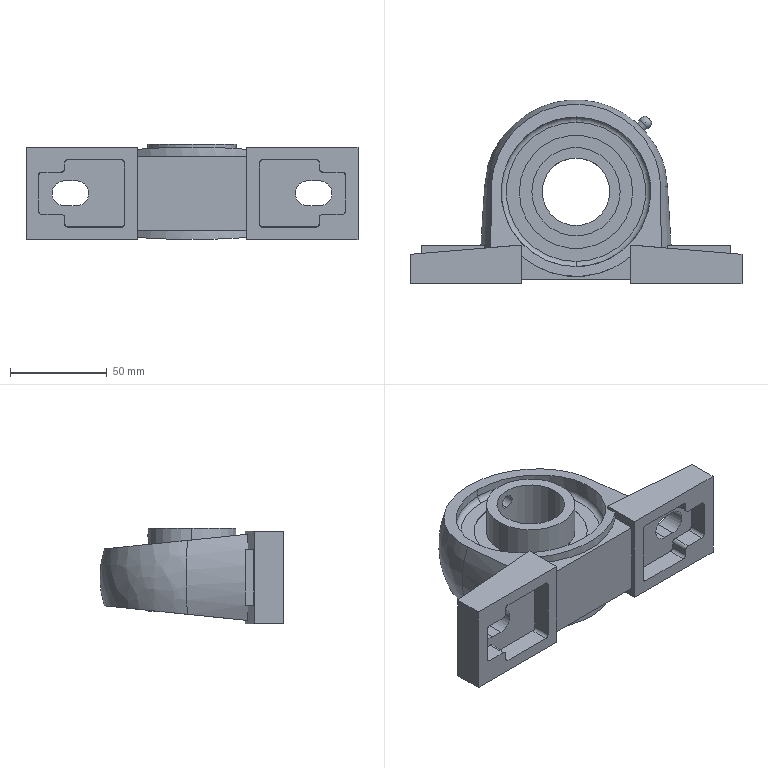Part | SolidWorks | features Revolution 5, Boss 3, Cut 3, RevCut 2, CirPattern 1, Extrusion 1, SweepCut 1 | 1 solid | 121 faces | box 172 x 95.2 x 49.4 mm | volume 226016 mm3 | plane 58 | cylinder 28 | cone 16 | sphere 8 | torus 8 | spline 3 | commonest cylinder face diameters 45.73 x6 58.72 x6 77.524 x6 13 x4 7.134 x2 35 x2